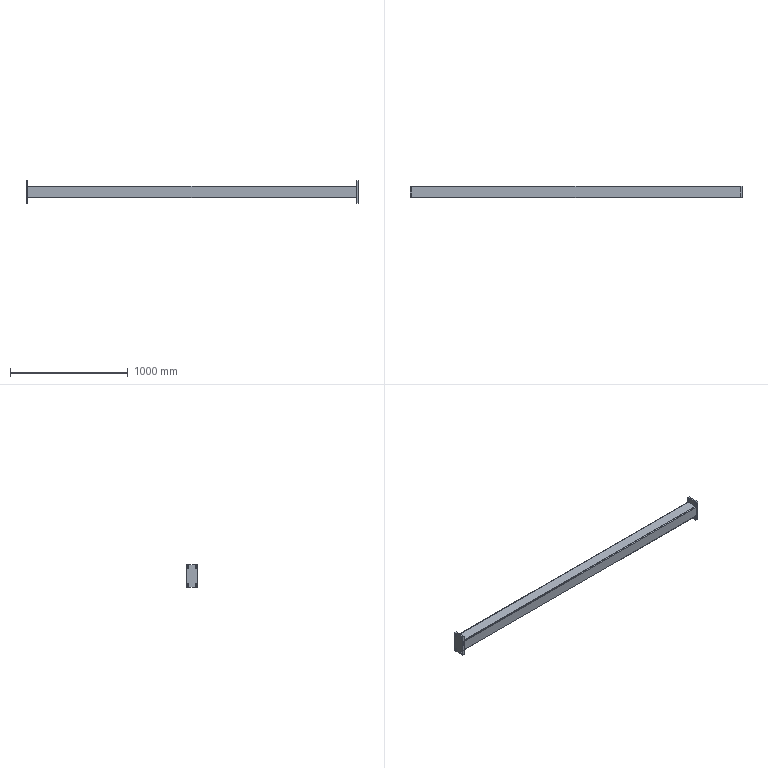Part | SolidWorks | features HoleWzd 1, ICE 1, MirrorSolid 1, WeldMemberFeat 1, WeldmentFeature 1 | 3 solids | 78 faces | box 2825 x 100 x 190 mm | volume 3924535 mm3 | plane 46 | cylinder 32 | commonest cylinder face diameters 13.5 x24 6.4 x4 12.8 x4